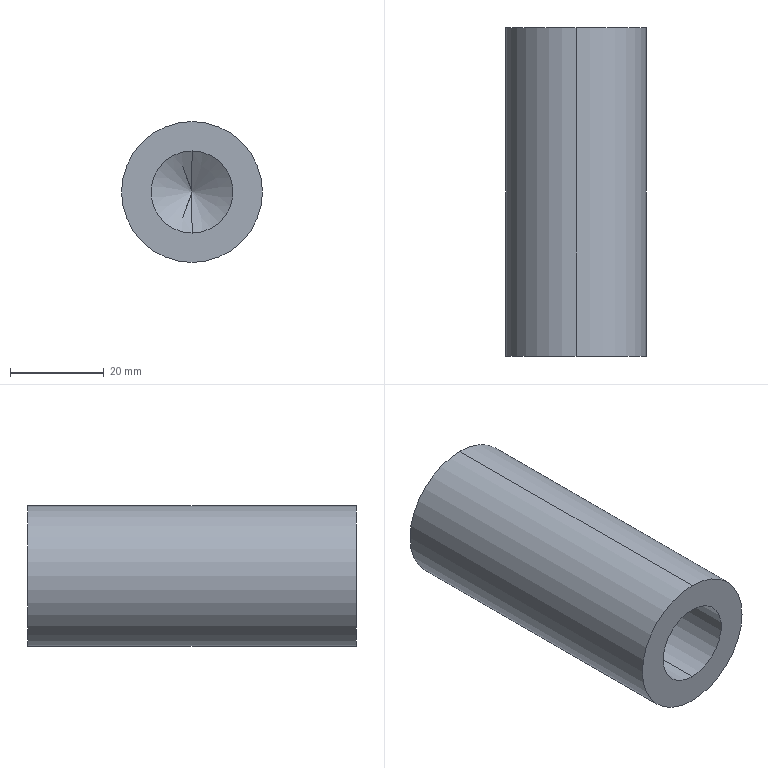Part | SolidWorks | features 3DProfileFeature 1, Extrusion 1, HoleWzd 1 | 1 solid | 8 faces | box 30 x 70 x 30 mm | volume 36431 mm3 | cylinder 4 | cone 2 | plane 2 | commonest cylinder face diameters 17.5 x2 30 x2
STEP:
#1=CARTESIAN_POINT('',(0.,17.5,8.75));
#2=VERTEX_POINT('',#1);
#3=CARTESIAN_POINT('',(0.,17.5,-8.75));
#4=VERTEX_POINT('',#3);
#5=CARTESIAN_POINT('',(0.,17.5,0.));
#6=DIRECTION('',(0.,-1.,0.));
#7=DIRECTION('',(0.,0.,-1.));
#8=AXIS2_PLACEMENT_3D('',#5,#6,#7);
#9=CIRCLE('',#8,8.75);
#10=EDGE_CURVE('',#2,#4,#9,.T.);
#11=ORIENTED_EDGE('',*,*,#10,.F.);
#12=CARTESIAN_POINT('',(0.,-35.,8.75));
#13=VERTEX_POINT('',#12);
#14=CARTESIAN_POINT('',(0.,-35.,8.75));
#15=DIRECTION('',(0.,-1.,0.));
#16=VECTOR('',#15,1000.);
#17=LINE('',#14,#16);
#18=EDGE_CURVE('',#2,#13,#17,.T.);
#19=ORIENTED_EDGE('',*,*,#18,.T.);
#20=CARTESIAN_POINT('',(0.,-35.,-8.75));
#21=VERTEX_POINT('',#20);
#22=CARTESIAN_POINT('',(0.,-35.,0.));
#23=DIRECTION('',(0.,-1.,0.));
#24=DIRECTION('',(0.,0.,-1.));
#25=AXIS2_PLACEMENT_3D('',#22,#23,#24);
#26=CIRCLE('',#25,8.75);
#27=EDGE_CURVE('',#13,#21,#26,.T.);
#28=ORIENTED_EDGE('',*,*,#27,.T.);
#29=CARTESIAN_POINT('',(0.,-35.,-8.75));
#30=DIRECTION('',(0.,-1.,0.));
#31=VECTOR('',#30,1000.);
#32=LINE('',#29,#31);
#33=EDGE_CURVE('',#4,#21,#32,.T.);
#34=ORIENTED_EDGE('',*,*,#33,.F.);
#35=EDGE_LOOP('',(#11,#19,#28,#34));
#36=FACE_OUTER_BOUND('',#35,.T.);
#37=CARTESIAN_POINT('',(0.,-35.,0.));
#38=DIRECTION('',(0.,-1.,0.));
#39=DIRECTION('',(0.,0.,-1.));
#40=AXIS2_PLACEMENT_3D('',#37,#38,#39);
#41=CYLINDRICAL_SURFACE('',#40,8.75);
#42=ADVANCED_FACE('',(#36),#41,.F.);
#43=CARTESIAN_POINT('',(0.,22.758,0.));
#44=VERTEX_POINT('',#43);
#45=CARTESIAN_POINT('',(0.,17.5,-8.75));
#46=DIRECTION('',(0.,-0.515,-0.8572));
#47=VECTOR('',#46,1000.);
#48=LINE('',#45,#47);
#49=EDGE_CURVE('',#44,#4,#48,.T.);
#50=ORIENTED_EDGE('',*,*,#49,.F.);
#51=CARTESIAN_POINT('',(0.,17.5,8.75));
#52=DIRECTION('',(0.,-0.515,0.8572));
#53=VECTOR('',#52,1000.);
#54=LINE('',#51,#53);
#55=EDGE_CURVE('',#44,#2,#54,.T.);
#56=ORIENTED_EDGE('',*,*,#55,.T.);
#57=ORIENTED_EDGE('',*,*,#10,.T.);
#58=EDGE_LOOP('',(#50,#56,#57));
#59=FACE_OUTER_BOUND('',#58,.T.);
#60=CARTESIAN_POINT('',(0.,17.5,0.));
#61=DIRECTION('',(0.,-1.,0.));
#62=DIRECTION('',(0.,0.,-1.));
#63=AXIS2_PLACEMENT_3D('',#60,#61,#62);
#64=CONICAL_SURFACE('',#63,8.75,1.03);
#65=ADVANCED_FACE('',(#59),#64,.F.);
#66=CARTESIAN_POINT('',(0.,35.,15.));
#67=VERTEX_POINT('',#66);
#68=CARTESIAN_POINT('',(0.,35.,-15.));
#69=VERTEX_POINT('',#68);
#70=CARTESIAN_POINT('',(0.,35.,0.));
#71=DIRECTION('',(0.,1.,0.));
#72=DIRECTION('',(0.,0.,1.));
#73=AXIS2_PLACEMENT_3D('',#70,#71,#72);
#74=CIRCLE('',#73,15.);
#75=EDGE_CURVE('',#67,#69,#74,.T.);
#76=ORIENTED_EDGE('',*,*,#75,.F.);
#77=CARTESIAN_POINT('',(0.,-35.,15.));
#78=VERTEX_POINT('',#77);
#79=CARTESIAN_POINT('',(0.,35.,15.));
#80=DIRECTION('',(0.,-1.,0.));
#81=VECTOR('',#80,1000.);
#82=LINE('',#79,#81);
#83=EDGE_CURVE('',#67,#78,#82,.T.);
#84=ORIENTED_EDGE('',*,*,#83,.T.);
#85=CARTESIAN_POINT('',(0.,-35.,-15.));
#86=VERTEX_POINT('',#85);
#87=CARTESIAN_POINT('',(0.,-35.,0.));
#88=DIRECTION('',(0.,1.,0.));
#89=DIRECTION('',(0.,0.,1.));
#90=AXIS2_PLACEMENT_3D('',#87,#88,#89);
#91=CIRCLE('',#90,15.);
#92=EDGE_CURVE('',#78,#86,#91,.T.);
#93=ORIENTED_EDGE('',*,*,#92,.T.);
#94=CARTESIAN_POINT('',(0.,35.,-15.));
#95=DIRECTION('',(0.,-1.,0.));
#96=VECTOR('',#95,1000.);
#97=LINE('',#94,#96);
#98=EDGE_CURVE('',#69,#86,#97,.T.);
#99=ORIENTED_EDGE('',*,*,#98,.F.);
#100=EDGE_LOOP('',(#76,#84,#93,#99));
#101=FACE_OUTER_BOUND('',#100,.T.);
#102=CARTESIAN_POINT('',(0.,35.,0.));
#103=DIRECTION('',(0.,-1.,0.));
#104=DIRECTION('',(0.,0.,-1.));
#105=AXIS2_PLACEMENT_3D('',#102,#103,#104);
#106=CYLINDRICAL_SURFACE('',#105,15.);
#107=ADVANCED_FACE('',(#101),#106,.T.);
#108=ORIENTED_EDGE('',*,*,#83,.F.);
#109=CARTESIAN_POINT('',(0.,35.,0.));
#110=DIRECTION('',(0.,1.,0.));
#111=DIRECTION('',(0.,0.,1.));
#112=AXIS2_PLACEMENT_3D('',#109,#110,#111);
#113=CIRCLE('',#112,15.);
#114=EDGE_CURVE('',#69,#67,#113,.T.);
#115=ORIENTED_EDGE('',*,*,#114,.F.);
#116=ORIENTED_EDGE('',*,*,#98,.T.);
#117=CARTESIAN_POINT('',(0.,-35.,0.));
#118=DIRECTION('',(0.,1.,0.));
#119=DIRECTION('',(0.,0.,1.));
#120=AXIS2_PLACEMENT_3D('',#117,#118,#119);
#121=CIRCLE('',#120,15.);
#122=EDGE_CURVE('',#86,#78,#121,.T.);
#123=ORIENTED_EDGE('',*,*,#122,.T.);
#124=EDGE_LOOP('',(#108,#115,#116,#123));
#125=FACE_OUTER_BOUND('',#124,.T.);
#126=CARTESIAN_POINT('',(0.,35.,0.));
#127=DIRECTION('',(0.,-1.,0.));
#128=DIRECTION('',(0.,0.,-1.));
#129=AXIS2_PLACEMENT_3D('',#126,#127,#128);
#130=CYLINDRICAL_SURFACE('',#129,15.);
#131=ADVANCED_FACE('',(#125),#130,.T.);
#132=ORIENTED_EDGE('',*,*,#114,.T.);
#133=ORIENTED_EDGE('',*,*,#75,.T.);
#134=EDGE_LOOP('',(#132,#133));
#135=FACE_OUTER_BOUND('',#134,.T.);
#136=CARTESIAN_POINT('',(0.,35.,0.));
#137=DIRECTION('',(0.,1.,0.));
#138=DIRECTION('',(0.,0.,1.));
#139=AXIS2_PLACEMENT_3D('',#136,#137,#138);
#140=PLANE('',#139);
#141=ADVANCED_FACE('',(#135),#140,.T.);
#142=CARTESIAN_POINT('',(0.,-35.,0.));
#143=DIRECTION('',(0.,-1.,0.));
#144=DIRECTION('',(0.,0.,-1.));
#145=AXIS2_PLACEMENT_3D('',#142,#143,#144);
#146=CIRCLE('',#145,8.75);
#147=EDGE_CURVE('',#21,#13,#146,.T.);
#148=ORIENTED_EDGE('',*,*,#147,.F.);
#149=ORIENTED_EDGE('',*,*,#27,.F.);
#150=EDGE_LOOP('',(#148,#149));
#151=FACE_BOUND('',#150,.T.);
#152=ORIENTED_EDGE('',*,*,#122,.F.);
#153=ORIENTED_EDGE('',*,*,#92,.F.);
#154=EDGE_LOOP('',(#152,#153));
#155=FACE_OUTER_BOUND('',#154,.T.);
#156=CARTESIAN_POINT('',(0.,-35.,0.));
#157=DIRECTION('',(0.,1.,0.));
#158=DIRECTION('',(0.,0.,1.));
#159=AXIS2_PLACEMENT_3D('',#156,#157,#158);
#160=PLANE('',#159);
#161=ADVANCED_FACE('',(#151,#155),#160,.F.);
#162=ORIENTED_EDGE('',*,*,#55,.F.);
#163=ORIENTED_EDGE('',*,*,#49,.T.);
#164=CARTESIAN_POINT('',(0.,17.5,0.));
#165=DIRECTION('',(0.,-1.,0.));
#166=DIRECTION('',(0.,0.,-1.));
#167=AXIS2_PLACEMENT_3D('',#164,#165,#166);
#168=CIRCLE('',#167,8.75);
#169=EDGE_CURVE('',#4,#2,#168,.T.);
#170=ORIENTED_EDGE('',*,*,#169,.T.);
#171=EDGE_LOOP('',(#162,#163,#170));
#172=FACE_OUTER_BOUND('',#171,.T.);
#173=CARTESIAN_POINT('',(0.,17.5,0.));
#174=DIRECTION('',(0.,-1.,0.));
#175=DIRECTION('',(0.,0.,-1.));
#176=AXIS2_PLACEMENT_3D('',#173,#174,#175);
#177=CONICAL_SURFACE('',#176,8.75,1.03);
#178=ADVANCED_FACE('',(#172),#177,.F.);
#179=ORIENTED_EDGE('',*,*,#18,.F.);
#180=ORIENTED_EDGE('',*,*,#169,.F.);
#181=ORIENTED_EDGE('',*,*,#33,.T.);
#182=ORIENTED_EDGE('',*,*,#147,.T.);
#183=EDGE_LOOP('',(#179,#180,#181,#182));
#184=FACE_OUTER_BOUND('',#183,.T.);
#185=CARTESIAN_POINT('',(0.,-35.,0.));
#186=DIRECTION('',(0.,-1.,0.));
#187=DIRECTION('',(0.,0.,-1.));
#188=AXIS2_PLACEMENT_3D('',#185,#186,#187);
#189=CYLINDRICAL_SURFACE('',#188,8.75);
#190=ADVANCED_FACE('',(#184),#189,.F.);
#191=CLOSED_SHELL('',(#42,#65,#107,#131,#141,#161,#178,#190));
#192=MANIFOLD_SOLID_BREP('',#191);
#193=CARTESIAN_POINT('',(0.,0.,0.));
#194=DIRECTION('',(0.,0.,1.));
#195=DIRECTION('',(1.,0.,0.));
#196=AXIS2_PLACEMENT_3D('',#193,#194,#195);
#197=(LENGTH_UNIT()NAMED_UNIT(*)SI_UNIT(.MILLI.,.METRE.));
#198=UNCERTAINTY_MEASURE_WITH_UNIT(LENGTH_MEASURE(0.00001),#197,'','');
#199=(NAMED_UNIT(*)PLANE_ANGLE_UNIT()SI_UNIT($,.RADIAN.));
#200=(NAMED_UNIT(*)SI_UNIT($,.STERADIAN.)SOLID_ANGLE_UNIT());
#201=(GEOMETRIC_REPRESENTATION_CONTEXT(3)GLOBAL_UNCERTAINTY_ASSIGNED_CONTEXT((#198))GLOBAL_UNIT_ASSIGNED_CONTEXT((#197,#199,#200))REPRESENTATION_CONTEXT('',''));
#202=ADVANCED_BREP_SHAPE_REPRESENTATION('',(#192,#196),#201);